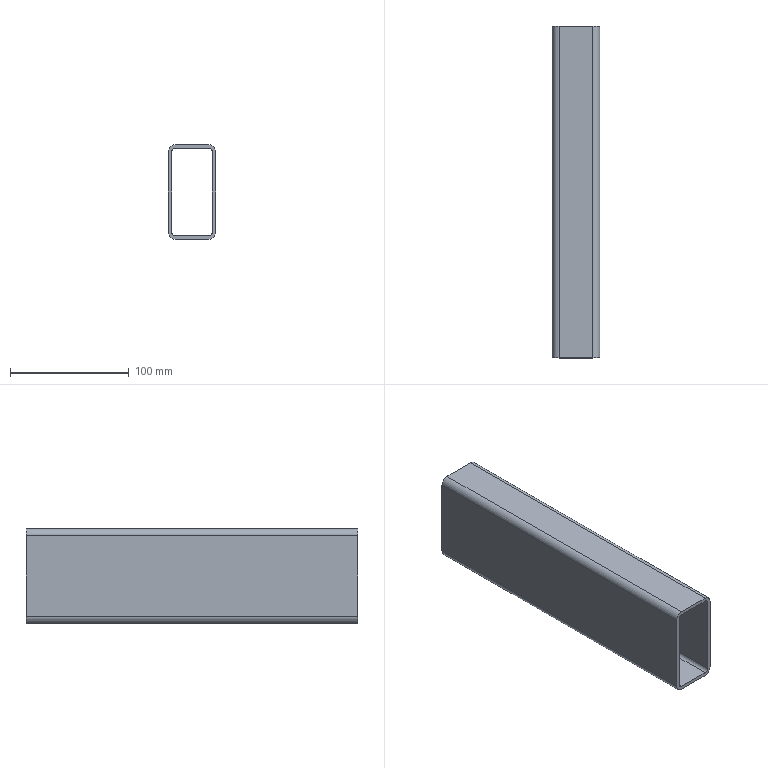Part | STEP file | SN10_002_008-06_TUBO_RETANGULAR | 1 solid | 18 faces | box 40 x 280 x 80 mm | volume 185030 mm3 | plane 10 | cylinder 8 | commonest cylinder face diameters 6 x4 12 x4
STEP:
#1=CARTESIAN_POINT('',(0.,0.,0.));
#2=DIRECTION('',(0.,0.,1.));
#3=DIRECTION('',(1.,0.,0.));
#4=AXIS2_PLACEMENT_3D('',#1,#2,#3);
#5=CARTESIAN_POINT('',(14.,-140.,40.));
#6=VERTEX_POINT('',#5);
#7=CARTESIAN_POINT('',(14.,140.,40.));
#8=VERTEX_POINT('',#7);
#9=CARTESIAN_POINT('',(14.,-140.,40.));
#10=DIRECTION('',(0.,1.,0.));
#11=VECTOR('',#10,1.);
#12=LINE('',#9,#11);
#13=CARTESIAN_POINT('',(14.,0.,34.));
#14=DIRECTION('',(0.,1.,0.));
#15=DIRECTION('',(0.,0.,1.));
#16=AXIS2_PLACEMENT_3D('',#13,#14,#15);
#17=CYLINDRICAL_SURFACE('',#16,6.);
#18=CARTESIAN_POINT('',(0.,-140.));
#19=DIRECTION('',(0.,1.));
#20=VECTOR('',#19,1.);
#21=LINE('',#18,#20);
#22=(GEOMETRIC_REPRESENTATION_CONTEXT(2)PARAMETRIC_REPRESENTATION_CONTEXT()REPRESENTATION_CONTEXT('',''));
#23=DEFINITIONAL_REPRESENTATION('',(#21),#22);
#24=PCURVE('',#17,#23);
#25=CARTESIAN_POINT('',(14.,0.,40.));
#26=DIRECTION('',(0.,0.,-1.));
#27=DIRECTION('',(-1.,0.,0.));
#28=AXIS2_PLACEMENT_3D('',#25,#26,#27);
#29=PLANE('',#28);
#30=CARTESIAN_POINT('',(0.,-140.));
#31=DIRECTION('',(0.,1.));
#32=VECTOR('',#31,1.);
#33=LINE('',#30,#32);
#34=(GEOMETRIC_REPRESENTATION_CONTEXT(2)PARAMETRIC_REPRESENTATION_CONTEXT()REPRESENTATION_CONTEXT('',''));
#35=DEFINITIONAL_REPRESENTATION('',(#33),#34);
#36=PCURVE('',#29,#35);
#37=SURFACE_CURVE('',#12,(#24,#36),.PCURVE_S1.);
#38=EDGE_CURVE('',#6,#8,#37,.T.);
#39=ORIENTED_EDGE('',*,*,#38,.F.);
#40=CARTESIAN_POINT('',(20.,-140.,34.));
#41=VERTEX_POINT('',#40);
#42=CARTESIAN_POINT('',(14.,-140.,34.));
#43=DIRECTION('',(0.,1.,0.));
#44=DIRECTION('',(1.,0.,0.));
#45=AXIS2_PLACEMENT_3D('',#42,#43,#44);
#46=CIRCLE('',#45,6.);
#47=CARTESIAN_POINT('',(-4.712,-140.));
#48=DIRECTION('',(1.,0.));
#49=VECTOR('',#48,1.);
#50=LINE('',#47,#49);
#51=(GEOMETRIC_REPRESENTATION_CONTEXT(2)PARAMETRIC_REPRESENTATION_CONTEXT()REPRESENTATION_CONTEXT('',''));
#52=DEFINITIONAL_REPRESENTATION('',(#50),#51);
#53=PCURVE('',#17,#52);
#54=CARTESIAN_POINT('',(0.,-140.,0.));
#55=DIRECTION('',(0.,1.,0.));
#56=DIRECTION('',(0.,0.,1.));
#57=AXIS2_PLACEMENT_3D('',#54,#55,#56);
#58=PLANE('',#57);
#59=CARTESIAN_POINT('',(34.,14.));
#60=DIRECTION('',(0.,1.));
#61=AXIS2_PLACEMENT_2D('',#59,#60);
#62=CIRCLE('',#61,6.);
#63=(GEOMETRIC_REPRESENTATION_CONTEXT(2)PARAMETRIC_REPRESENTATION_CONTEXT()REPRESENTATION_CONTEXT('',''));
#64=DEFINITIONAL_REPRESENTATION('',(#62),#63);
#65=PCURVE('',#58,#64);
#66=SURFACE_CURVE('',#46,(#53,#65),.PCURVE_S1.);
#67=EDGE_CURVE('',#6,#41,#66,.T.);
#68=ORIENTED_EDGE('',*,*,#67,.T.);
#69=CARTESIAN_POINT('',(20.,140.,34.));
#70=VERTEX_POINT('',#69);
#71=CARTESIAN_POINT('',(20.,-140.,34.));
#72=DIRECTION('',(0.,1.,0.));
#73=VECTOR('',#72,1.);
#74=LINE('',#71,#73);
#75=CARTESIAN_POINT('',(1.571,-140.));
#76=DIRECTION('',(0.,1.));
#77=VECTOR('',#76,1.);
#78=LINE('',#75,#77);
#79=(GEOMETRIC_REPRESENTATION_CONTEXT(2)PARAMETRIC_REPRESENTATION_CONTEXT()REPRESENTATION_CONTEXT('',''));
#80=DEFINITIONAL_REPRESENTATION('',(#78),#79);
#81=PCURVE('',#17,#80);
#82=CARTESIAN_POINT('',(20.,0.,-34.));
#83=DIRECTION('',(-1.,0.,0.));
#84=DIRECTION('',(0.,0.,1.));
#85=AXIS2_PLACEMENT_3D('',#82,#83,#84);
#86=PLANE('',#85);
#87=CARTESIAN_POINT('',(68.,-140.));
#88=DIRECTION('',(0.,1.));
#89=VECTOR('',#88,1.);
#90=LINE('',#87,#89);
#91=(GEOMETRIC_REPRESENTATION_CONTEXT(2)PARAMETRIC_REPRESENTATION_CONTEXT()REPRESENTATION_CONTEXT('',''));
#92=DEFINITIONAL_REPRESENTATION('',(#90),#91);
#93=PCURVE('',#86,#92);
#94=SURFACE_CURVE('',#74,(#81,#93),.PCURVE_S1.);
#95=EDGE_CURVE('',#41,#70,#94,.T.);
#96=ORIENTED_EDGE('',*,*,#95,.T.);
#97=CARTESIAN_POINT('',(14.,140.,34.));
#98=DIRECTION('',(0.,1.,0.));
#99=DIRECTION('',(1.,0.,0.));
#100=AXIS2_PLACEMENT_3D('',#97,#98,#99);
#101=CIRCLE('',#100,6.);
#102=CARTESIAN_POINT('',(-4.712,140.));
#103=DIRECTION('',(1.,0.));
#104=VECTOR('',#103,1.);
#105=LINE('',#102,#104);
#106=(GEOMETRIC_REPRESENTATION_CONTEXT(2)PARAMETRIC_REPRESENTATION_CONTEXT()REPRESENTATION_CONTEXT('',''));
#107=DEFINITIONAL_REPRESENTATION('',(#105),#106);
#108=PCURVE('',#17,#107);
#109=CARTESIAN_POINT('',(0.,140.,0.));
#110=DIRECTION('',(0.,1.,0.));
#111=DIRECTION('',(0.,0.,1.));
#112=AXIS2_PLACEMENT_3D('',#109,#110,#111);
#113=PLANE('',#112);
#114=CARTESIAN_POINT('',(34.,14.));
#115=DIRECTION('',(0.,1.));
#116=AXIS2_PLACEMENT_2D('',#114,#115);
#117=CIRCLE('',#116,6.);
#118=(GEOMETRIC_REPRESENTATION_CONTEXT(2)PARAMETRIC_REPRESENTATION_CONTEXT()REPRESENTATION_CONTEXT('',''));
#119=DEFINITIONAL_REPRESENTATION('',(#117),#118);
#120=PCURVE('',#113,#119);
#121=SURFACE_CURVE('',#101,(#108,#120),.PCURVE_S1.);
#122=EDGE_CURVE('',#8,#70,#121,.T.);
#123=ORIENTED_EDGE('',*,*,#122,.F.);
#124=EDGE_LOOP('',(#39,#68,#96,#123));
#125=FACE_BOUND('',#124,.T.);
#126=ADVANCED_FACE('',(#125),#17,.T.);
#127=ORIENTED_EDGE('',*,*,#95,.F.);
#128=CARTESIAN_POINT('',(20.,-140.,-34.));
#129=VERTEX_POINT('',#128);
#130=CARTESIAN_POINT('',(20.,-140.,-34.));
#131=DIRECTION('',(0.,0.,1.));
#132=VECTOR('',#131,1.);
#133=LINE('',#130,#132);
#134=CARTESIAN_POINT('',(0.,-140.));
#135=DIRECTION('',(1.,0.));
#136=VECTOR('',#135,1.);
#137=LINE('',#134,#136);
#138=(GEOMETRIC_REPRESENTATION_CONTEXT(2)PARAMETRIC_REPRESENTATION_CONTEXT()REPRESENTATION_CONTEXT('',''));
#139=DEFINITIONAL_REPRESENTATION('',(#137),#138);
#140=PCURVE('',#86,#139);
#141=CARTESIAN_POINT('',(-34.,20.));
#142=DIRECTION('',(1.,0.));
#143=VECTOR('',#142,1.);
#144=LINE('',#141,#143);
#145=(GEOMETRIC_REPRESENTATION_CONTEXT(2)PARAMETRIC_REPRESENTATION_CONTEXT()REPRESENTATION_CONTEXT('',''));
#146=DEFINITIONAL_REPRESENTATION('',(#144),#145);
#147=PCURVE('',#58,#146);
#148=SURFACE_CURVE('',#133,(#140,#147),.PCURVE_S1.);
#149=EDGE_CURVE('',#129,#41,#148,.T.);
#150=ORIENTED_EDGE('',*,*,#149,.F.);
#151=CARTESIAN_POINT('',(20.,140.,-34.));
#152=VERTEX_POINT('',#151);
#153=CARTESIAN_POINT('',(20.,-140.,-34.));
#154=DIRECTION('',(0.,1.,0.));
#155=VECTOR('',#154,1.);
#156=LINE('',#153,#155);
#157=CARTESIAN_POINT('',(0.,-140.));
#158=DIRECTION('',(0.,1.));
#159=VECTOR('',#158,1.);
#160=LINE('',#157,#159);
#161=(GEOMETRIC_REPRESENTATION_CONTEXT(2)PARAMETRIC_REPRESENTATION_CONTEXT()REPRESENTATION_CONTEXT('',''));
#162=DEFINITIONAL_REPRESENTATION('',(#160),#161);
#163=PCURVE('',#86,#162);
#164=CARTESIAN_POINT('',(14.,0.,-34.));
#165=DIRECTION('',(0.,1.,0.));
#166=DIRECTION('',(1.,0.,0.));
#167=AXIS2_PLACEMENT_3D('',#164,#165,#166);
#168=CYLINDRICAL_SURFACE('',#167,6.);
#169=CARTESIAN_POINT('',(0.,-140.));
#170=DIRECTION('',(0.,1.));
#171=VECTOR('',#170,1.);
#172=LINE('',#169,#171);
#173=(GEOMETRIC_REPRESENTATION_CONTEXT(2)PARAMETRIC_REPRESENTATION_CONTEXT()REPRESENTATION_CONTEXT('',''));
#174=DEFINITIONAL_REPRESENTATION('',(#172),#173);
#175=PCURVE('',#168,#174);
#176=SURFACE_CURVE('',#156,(#163,#175),.PCURVE_S1.);
#177=EDGE_CURVE('',#129,#152,#176,.T.);
#178=ORIENTED_EDGE('',*,*,#177,.T.);
#179=CARTESIAN_POINT('',(20.,140.,-34.));
#180=DIRECTION('',(0.,0.,1.));
#181=VECTOR('',#180,1.);
#182=LINE('',#179,#181);
#183=CARTESIAN_POINT('',(0.,140.));
#184=DIRECTION('',(1.,0.));
#185=VECTOR('',#184,1.);
#186=LINE('',#183,#185);
#187=(GEOMETRIC_REPRESENTATION_CONTEXT(2)PARAMETRIC_REPRESENTATION_CONTEXT()REPRESENTATION_CONTEXT('',''));
#188=DEFINITIONAL_REPRESENTATION('',(#186),#187);
#189=PCURVE('',#86,#188);
#190=CARTESIAN_POINT('',(-34.,20.));
#191=DIRECTION('',(1.,0.));
#192=VECTOR('',#191,1.);
#193=LINE('',#190,#192);
#194=(GEOMETRIC_REPRESENTATION_CONTEXT(2)PARAMETRIC_REPRESENTATION_CONTEXT()REPRESENTATION_CONTEXT('',''));
#195=DEFINITIONAL_REPRESENTATION('',(#193),#194);
#196=PCURVE('',#113,#195);
#197=SURFACE_CURVE('',#182,(#189,#196),.PCURVE_S1.);
#198=EDGE_CURVE('',#152,#70,#197,.T.);
#199=ORIENTED_EDGE('',*,*,#198,.T.);
#200=EDGE_LOOP('',(#127,#150,#178,#199));
#201=FACE_BOUND('',#200,.T.);
#202=ADVANCED_FACE('',(#201),#86,.F.);
#203=ORIENTED_EDGE('',*,*,#177,.F.);
#204=CARTESIAN_POINT('',(14.,-140.,-40.));
#205=VERTEX_POINT('',#204);
#206=CARTESIAN_POINT('',(14.,-140.,-34.));
#207=DIRECTION('',(0.,1.,0.));
#208=DIRECTION('',(1.,0.,0.));
#209=AXIS2_PLACEMENT_3D('',#206,#207,#208);
#210=CIRCLE('',#209,6.);
#211=CARTESIAN_POINT('',(0.,-140.));
#212=DIRECTION('',(1.,0.));
#213=VECTOR('',#212,1.);
#214=LINE('',#211,#213);
#215=(GEOMETRIC_REPRESENTATION_CONTEXT(2)PARAMETRIC_REPRESENTATION_CONTEXT()REPRESENTATION_CONTEXT('',''));
#216=DEFINITIONAL_REPRESENTATION('',(#214),#215);
#217=PCURVE('',#168,#216);
#218=CARTESIAN_POINT('',(-34.,14.));
#219=DIRECTION('',(0.,1.));
#220=AXIS2_PLACEMENT_2D('',#218,#219);
#221=CIRCLE('',#220,6.);
#222=(GEOMETRIC_REPRESENTATION_CONTEXT(2)PARAMETRIC_REPRESENTATION_CONTEXT()REPRESENTATION_CONTEXT('',''));
#223=DEFINITIONAL_REPRESENTATION('',(#221),#222);
#224=PCURVE('',#58,#223);
#225=SURFACE_CURVE('',#210,(#217,#224),.PCURVE_S1.);
#226=EDGE_CURVE('',#129,#205,#225,.T.);
#227=ORIENTED_EDGE('',*,*,#226,.T.);
#228=CARTESIAN_POINT('',(14.,140.,-40.));
#229=VERTEX_POINT('',#228);
#230=CARTESIAN_POINT('',(14.,-140.,-40.));
#231=DIRECTION('',(0.,1.,0.));
#232=VECTOR('',#231,1.);
#233=LINE('',#230,#232);
#234=CARTESIAN_POINT('',(1.571,-140.));
#235=DIRECTION('',(0.,1.));
#236=VECTOR('',#235,1.);
#237=LINE('',#234,#236);
#238=(GEOMETRIC_REPRESENTATION_CONTEXT(2)PARAMETRIC_REPRESENTATION_CONTEXT()REPRESENTATION_CONTEXT('',''));
#239=DEFINITIONAL_REPRESENTATION('',(#237),#238);
#240=PCURVE('',#168,#239);
#241=CARTESIAN_POINT('',(-14.,0.,-40.));
#242=DIRECTION('',(0.,0.,1.));
#243=DIRECTION('',(1.,0.,0.));
#244=AXIS2_PLACEMENT_3D('',#241,#242,#243);
#245=PLANE('',#244);
#246=CARTESIAN_POINT('',(28.,-140.));
#247=DIRECTION('',(0.,1.));
#248=VECTOR('',#247,1.);
#249=LINE('',#246,#248);
#250=(GEOMETRIC_REPRESENTATION_CONTEXT(2)PARAMETRIC_REPRESENTATION_CONTEXT()REPRESENTATION_CONTEXT('',''));
#251=DEFINITIONAL_REPRESENTATION('',(#249),#250);
#252=PCURVE('',#245,#251);
#253=SURFACE_CURVE('',#233,(#240,#252),.PCURVE_S1.);
#254=EDGE_CURVE('',#205,#229,#253,.T.);
#255=ORIENTED_EDGE('',*,*,#254,.T.);
#256=CARTESIAN_POINT('',(14.,140.,-34.));
#257=DIRECTION('',(0.,1.,0.));
#258=DIRECTION('',(1.,0.,0.));
#259=AXIS2_PLACEMENT_3D('',#256,#257,#258);
#260=CIRCLE('',#259,6.);
#261=CARTESIAN_POINT('',(0.,140.));
#262=DIRECTION('',(1.,0.));
#263=VECTOR('',#262,1.);
#264=LINE('',#261,#263);
#265=(GEOMETRIC_REPRESENTATION_CONTEXT(2)PARAMETRIC_REPRESENTATION_CONTEXT()REPRESENTATION_CONTEXT('',''));
#266=DEFINITIONAL_REPRESENTATION('',(#264),#265);
#267=PCURVE('',#168,#266);
#268=CARTESIAN_POINT('',(-34.,14.));
#269=DIRECTION('',(0.,1.));
#270=AXIS2_PLACEMENT_2D('',#268,#269);
#271=CIRCLE('',#270,6.);
#272=(GEOMETRIC_REPRESENTATION_CONTEXT(2)PARAMETRIC_REPRESENTATION_CONTEXT()REPRESENTATION_CONTEXT('',''));
#273=DEFINITIONAL_REPRESENTATION('',(#271),#272);
#274=PCURVE('',#113,#273);
#275=SURFACE_CURVE('',#260,(#267,#274),.PCURVE_S1.);
#276=EDGE_CURVE('',#152,#229,#275,.T.);
#277=ORIENTED_EDGE('',*,*,#276,.F.);
#278=EDGE_LOOP('',(#203,#227,#255,#277));
#279=FACE_BOUND('',#278,.T.);
#280=ADVANCED_FACE('',(#279),#168,.T.);
#281=ORIENTED_EDGE('',*,*,#254,.F.);
#282=CARTESIAN_POINT('',(-14.,-140.,-40.));
#283=VERTEX_POINT('',#282);
#284=CARTESIAN_POINT('',(-14.,-140.,-40.));
#285=DIRECTION('',(1.,0.,0.));
#286=VECTOR('',#285,1.);
#287=LINE('',#284,#286);
#288=CARTESIAN_POINT('',(0.,-140.));
#289=DIRECTION('',(1.,0.));
#290=VECTOR('',#289,1.);
#291=LINE('',#288,#290);
#292=(GEOMETRIC_REPRESENTATION_CONTEXT(2)PARAMETRIC_REPRESENTATION_CONTEXT()REPRESENTATION_CONTEXT('',''));
#293=DEFINITIONAL_REPRESENTATION('',(#291),#292);
#294=PCURVE('',#245,#293);
#295=CARTESIAN_POINT('',(-40.,-14.));
#296=DIRECTION('',(0.,1.));
#297=VECTOR('',#296,1.);
#298=LINE('',#295,#297);
#299=(GEOMETRIC_REPRESENTATION_CONTEXT(2)PARAMETRIC_REPRESENTATION_CONTEXT()REPRESENTATION_CONTEXT('',''));
#300=DEFINITIONAL_REPRESENTATION('',(#298),#299);
#301=PCURVE('',#58,#300);
#302=SURFACE_CURVE('',#287,(#294,#301),.PCURVE_S1.);
#303=EDGE_CURVE('',#283,#205,#302,.T.);
#304=ORIENTED_EDGE('',*,*,#303,.F.);
#305=CARTESIAN_POINT('',(-14.,140.,-40.));
#306=VERTEX_POINT('',#305);
#307=CARTESIAN_POINT('',(-14.,-140.,-40.));
#308=DIRECTION('',(0.,1.,0.));
#309=VECTOR('',#308,1.);
#310=LINE('',#307,#309);
#311=CARTESIAN_POINT('',(0.,-140.));
#312=DIRECTION('',(0.,1.));
#313=VECTOR('',#312,1.);
#314=LINE('',#311,#313);
#315=(GEOMETRIC_REPRESENTATION_CONTEXT(2)PARAMETRIC_REPRESENTATION_CONTEXT()REPRESENTATION_CONTEXT('',''));
#316=DEFINITIONAL_REPRESENTATION('',(#314),#315);
#317=PCURVE('',#245,#316);
#318=CARTESIAN_POINT('',(-14.,0.,-34.));
#319=DIRECTION('',(0.,1.,0.));
#320=DIRECTION('',(0.,0.,-1.));
#321=AXIS2_PLACEMENT_3D('',#318,#319,#320);
#322=CYLINDRICAL_SURFACE('',#321,6.);
#323=CARTESIAN_POINT('',(0.,-140.));
#324=DIRECTION('',(0.,1.));
#325=VECTOR('',#324,1.);
#326=LINE('',#323,#325);
#327=(GEOMETRIC_REPRESENTATION_CONTEXT(2)PARAMETRIC_REPRESENTATION_CONTEXT()REPRESENTATION_CONTEXT('',''));
#328=DEFINITIONAL_REPRESENTATION('',(#326),#327);
#329=PCURVE('',#322,#328);
#330=SURFACE_CURVE('',#310,(#317,#329),.PCURVE_S1.);
#331=EDGE_CURVE('',#283,#306,#330,.T.);
#332=ORIENTED_EDGE('',*,*,#331,.T.);
#333=CARTESIAN_POINT('',(-14.,140.,-40.));
#334=DIRECTION('',(1.,0.,0.));
#335=VECTOR('',#334,1.);
#336=LINE('',#333,#335);
#337=CARTESIAN_POINT('',(0.,140.));
#338=DIRECTION('',(1.,0.));
#339=VECTOR('',#338,1.);
#340=LINE('',#337,#339);
#341=(GEOMETRIC_REPRESENTATION_CONTEXT(2)PARAMETRIC_REPRESENTATION_CONTEXT()REPRESENTATION_CONTEXT('',''));
#342=DEFINITIONAL_REPRESENTATION('',(#340),#341);
#343=PCURVE('',#245,#342);
#344=CARTESIAN_POINT('',(-40.,-14.));
#345=DIRECTION('',(0.,1.));
#346=VECTOR('',#345,1.);
#347=LINE('',#344,#346);
#348=(GEOMETRIC_REPRESENTATION_CONTEXT(2)PARAMETRIC_REPRESENTATION_CONTEXT()REPRESENTATION_CONTEXT('',''));
#349=DEFINITIONAL_REPRESENTATION('',(#347),#348);
#350=PCURVE('',#113,#349);
#351=SURFACE_CURVE('',#336,(#343,#350),.PCURVE_S1.);
#352=EDGE_CURVE('',#306,#229,#351,.T.);
#353=ORIENTED_EDGE('',*,*,#352,.T.);
#354=EDGE_LOOP('',(#281,#304,#332,#353));
#355=FACE_BOUND('',#354,.T.);
#356=ADVANCED_FACE('',(#355),#245,.F.);
#357=ORIENTED_EDGE('',*,*,#331,.F.);
#358=CARTESIAN_POINT('',(-20.,-140.,-34.));
#359=VERTEX_POINT('',#358);
#360=CARTESIAN_POINT('',(-14.,-140.,-34.));
#361=DIRECTION('',(0.,1.,0.));
#362=DIRECTION('',(1.,0.,0.));
#363=AXIS2_PLACEMENT_3D('',#360,#361,#362);
#364=CIRCLE('',#363,6.);
#365=CARTESIAN_POINT('',(-1.571,-140.));
#366=DIRECTION('',(1.,0.));
#367=VECTOR('',#366,1.);
#368=LINE('',#365,#367);
#369=(GEOMETRIC_REPRESENTATION_CONTEXT(2)PARAMETRIC_REPRESENTATION_CONTEXT()REPRESENTATION_CONTEXT('',''));
#370=DEFINITIONAL_REPRESENTATION('',(#368),#369);
#371=PCURVE('',#322,#370);
#372=CARTESIAN_POINT('',(-34.,-14.));
#373=DIRECTION('',(0.,1.));
#374=AXIS2_PLACEMENT_2D('',#372,#373);
#375=CIRCLE('',#374,6.);
#376=(GEOMETRIC_REPRESENTATION_CONTEXT(2)PARAMETRIC_REPRESENTATION_CONTEXT()REPRESENTATION_CONTEXT('',''));
#377=DEFINITIONAL_REPRESENTATION('',(#375),#376);
#378=PCURVE('',#58,#377);
#379=SURFACE_CURVE('',#364,(#371,#378),.PCURVE_S1.);
#380=EDGE_CURVE('',#283,#359,#379,.T.);
#381=ORIENTED_EDGE('',*,*,#380,.T.);
#382=CARTESIAN_POINT('',(-20.,140.,-34.));
#383=VERTEX_POINT('',#382);
#384=CARTESIAN_POINT('',(-20.,-140.,-34.));
#385=DIRECTION('',(0.,1.,0.));
#386=VECTOR('',#385,1.);
#387=LINE('',#384,#386);
#388=CARTESIAN_POINT('',(1.571,-140.));
#389=DIRECTION('',(0.,1.));
#390=VECTOR('',#389,1.);
#391=LINE('',#388,#390);
#392=(GEOMETRIC_REPRESENTATION_CONTEXT(2)PARAMETRIC_REPRESENTATION_CONTEXT()REPRESENTATION_CONTEXT('',''));
#393=DEFINITIONAL_REPRESENTATION('',(#391),#392);
#394=PCURVE('',#322,#393);
#395=CARTESIAN_POINT('',(-20.,0.,34.));
#396=DIRECTION('',(1.,0.,0.));
#397=DIRECTION('',(0.,0.,-1.));
#398=AXIS2_PLACEMENT_3D('',#395,#396,#397);
#399=PLANE('',#398);
#400=CARTESIAN_POINT('',(68.,-140.));
#401=DIRECTION('',(0.,1.));
#402=VECTOR('',#401,1.);
#403=LINE('',#400,#402);
#404=(GEOMETRIC_REPRESENTATION_CONTEXT(2)PARAMETRIC_REPRESENTATION_CONTEXT()REPRESENTATION_CONTEXT('',''));
#405=DEFINITIONAL_REPRESENTATION('',(#403),#404);
#406=PCURVE('',#399,#405);
#407=SURFACE_CURVE('',#387,(#394,#406),.PCURVE_S1.);
#408=EDGE_CURVE('',#359,#383,#407,.T.);
#409=ORIENTED_EDGE('',*,*,#408,.T.);
#410=CARTESIAN_POINT('',(-14.,140.,-34.));
#411=DIRECTION('',(0.,1.,0.));
#412=DIRECTION('',(1.,0.,0.));
#413=AXIS2_PLACEMENT_3D('',#410,#411,#412);
#414=CIRCLE('',#413,6.);
#415=CARTESIAN_POINT('',(-1.571,140.));
#416=DIRECTION('',(1.,0.));
#417=VECTOR('',#416,1.);
#418=LINE('',#415,#417);
#419=(GEOMETRIC_REPRESENTATION_CONTEXT(2)PARAMETRIC_REPRESENTATION_CONTEXT()REPRESENTATION_CONTEXT('',''));
#420=DEFINITIONAL_REPRESENTATION('',(#418),#419);
#421=PCURVE('',#322,#420);
#422=CARTESIAN_POINT('',(-34.,-14.));
#423=DIRECTION('',(0.,1.));
#424=AXIS2_PLACEMENT_2D('',#422,#423);
#425=CIRCLE('',#424,6.);
#426=(GEOMETRIC_REPRESENTATION_CONTEXT(2)PARAMETRIC_REPRESENTATION_CONTEXT()REPRESENTATION_CONTEXT('',''));
#427=DEFINITIONAL_REPRESENTATION('',(#425),#426);
#428=PCURVE('',#113,#427);
#429=SURFACE_CURVE('',#414,(#421,#428),.PCURVE_S1.);
#430=EDGE_CURVE('',#306,#383,#429,.T.);
#431=ORIENTED_EDGE('',*,*,#430,.F.);
#432=EDGE_LOOP('',(#357,#381,#409,#431));
#433=FACE_BOUND('',#432,.T.);
#434=ADVANCED_FACE('',(#433),#322,.T.);
#435=ORIENTED_EDGE('',*,*,#408,.F.);
#436=CARTESIAN_POINT('',(-20.,-140.,34.));
#437=VERTEX_POINT('',#436);
#438=CARTESIAN_POINT('',(-20.,-140.,34.));
#439=DIRECTION('',(0.,0.,-1.));
#440=VECTOR('',#439,1.);
#441=LINE('',#438,#440);
#442=CARTESIAN_POINT('',(0.,-140.));
#443=DIRECTION('',(1.,0.));
#444=VECTOR('',#443,1.);
#445=LINE('',#442,#444);
#446=(GEOMETRIC_REPRESENTATION_CONTEXT(2)PARAMETRIC_REPRESENTATION_CONTEXT()REPRESENTATION_CONTEXT('',''));
#447=DEFINITIONAL_REPRESENTATION('',(#445),#446);
#448=PCURVE('',#399,#447);
#449=CARTESIAN_POINT('',(34.,-20.));
#450=DIRECTION('',(-1.,0.));
#451=VECTOR('',#450,1.);
#452=LINE('',#449,#451);
#453=(GEOMETRIC_REPRESENTATION_CONTEXT(2)PARAMETRIC_REPRESENTATION_CONTEXT()REPRESENTATION_CONTEXT('',''));
#454=DEFINITIONAL_REPRESENTATION('',(#452),#453);
#455=PCURVE('',#58,#454);
#456=SURFACE_CURVE('',#441,(#448,#455),.PCURVE_S1.);
#457=EDGE_CURVE('',#437,#359,#456,.T.);
#458=ORIENTED_EDGE('',*,*,#457,.F.);
#459=CARTESIAN_POINT('',(-20.,140.,34.));
#460=VERTEX_POINT('',#459);
#461=CARTESIAN_POINT('',(-20.,-140.,34.));
#462=DIRECTION('',(0.,1.,0.));
#463=VECTOR('',#462,1.);
#464=LINE('',#461,#463);
#465=CARTESIAN_POINT('',(0.,-140.));
#466=DIRECTION('',(0.,1.));
#467=VECTOR('',#466,1.);
#468=LINE('',#465,#467);
#469=(GEOMETRIC_REPRESENTATION_CONTEXT(2)PARAMETRIC_REPRESENTATION_CONTEXT()REPRESENTATION_CONTEXT('',''));
#470=DEFINITIONAL_REPRESENTATION('',(#468),#469);
#471=PCURVE('',#399,#470);
#472=CARTESIAN_POINT('',(-14.,0.,34.));
#473=DIRECTION('',(0.,1.,0.));
#474=DIRECTION('',(-1.,0.,0.));
#475=AXIS2_PLACEMENT_3D('',#472,#473,#474);
#476=CYLINDRICAL_SURFACE('',#475,6.);
#477=CARTESIAN_POINT('',(0.,-140.));
#478=DIRECTION('',(0.,1.));
#479=VECTOR('',#478,1.);
#480=LINE('',#477,#479);
#481=(GEOMETRIC_REPRESENTATION_CONTEXT(2)PARAMETRIC_REPRESENTATION_CONTEXT()REPRESENTATION_CONTEXT('',''));
#482=DEFINITIONAL_REPRESENTATION('',(#480),#481);
#483=PCURVE('',#476,#482);
#484=SURFACE_CURVE('',#464,(#471,#483),.PCURVE_S1.);
#485=EDGE_CURVE('',#437,#460,#484,.T.);
#486=ORIENTED_EDGE('',*,*,#485,.T.);
#487=CARTESIAN_POINT('',(-20.,140.,34.));
#488=DIRECTION('',(0.,0.,-1.));
#489=VECTOR('',#488,1.);
#490=LINE('',#487,#489);
#491=CARTESIAN_POINT('',(0.,140.));
#492=DIRECTION('',(1.,0.));
#493=VECTOR('',#492,1.);
#494=LINE('',#491,#493);
#495=(GEOMETRIC_REPRESENTATION_CONTEXT(2)PARAMETRIC_REPRESENTATION_CONTEXT()REPRESENTATION_CONTEXT('',''));
#496=DEFINITIONAL_REPRESENTATION('',(#494),#495);
#497=PCURVE('',#399,#496);
#498=CARTESIAN_POINT('',(34.,-20.));
#499=DIRECTION('',(-1.,0.));
#500=VECTOR('',#499,1.);
#501=LINE('',#498,#500);
#502=(GEOMETRIC_REPRESENTATION_CONTEXT(2)PARAMETRIC_REPRESENTATION_CONTEXT()REPRESENTATION_CONTEXT('',''));
#503=DEFINITIONAL_REPRESENTATION('',(#501),#502);
#504=PCURVE('',#113,#503);
#505=SURFACE_CURVE('',#490,(#497,#504),.PCURVE_S1.);
#506=EDGE_CURVE('',#460,#383,#505,.T.);
#507=ORIENTED_EDGE('',*,*,#506,.T.);
#508=EDGE_LOOP('',(#435,#458,#486,#507));
#509=FACE_BOUND('',#508,.T.);
#510=ADVANCED_FACE('',(#509),#399,.F.);
#511=ORIENTED_EDGE('',*,*,#485,.F.);
#512=CARTESIAN_POINT('',(-14.,-140.,40.));
#513=VERTEX_POINT('',#512);
#514=CARTESIAN_POINT('',(-14.,-140.,34.));
#515=DIRECTION('',(0.,1.,0.));
#516=DIRECTION('',(1.,0.,0.));
#517=AXIS2_PLACEMENT_3D('',#514,#515,#516);
#518=CIRCLE('',#517,6.);
#519=CARTESIAN_POINT('',(-3.142,-140.));
#520=DIRECTION('',(1.,0.));
#521=VECTOR('',#520,1.);
#522=LINE('',#519,#521);
#523=(GEOMETRIC_REPRESENTATION_CONTEXT(2)PARAMETRIC_REPRESENTATION_CONTEXT()REPRESENTATION_CONTEXT('',''));
#524=DEFINITIONAL_REPRESENTATION('',(#522),#523);
#525=PCURVE('',#476,#524);
#526=CARTESIAN_POINT('',(34.,-14.));
#527=DIRECTION('',(0.,1.));
#528=AXIS2_PLACEMENT_2D('',#526,#527);
#529=CIRCLE('',#528,6.);
#530=(GEOMETRIC_REPRESENTATION_CONTEXT(2)PARAMETRIC_REPRESENTATION_CONTEXT()REPRESENTATION_CONTEXT('',''));
#531=DEFINITIONAL_REPRESENTATION('',(#529),#530);
#532=PCURVE('',#58,#531);
#533=SURFACE_CURVE('',#518,(#525,#532),.PCURVE_S1.);
#534=EDGE_CURVE('',#437,#513,#533,.T.);
#535=ORIENTED_EDGE('',*,*,#534,.T.);
#536=CARTESIAN_POINT('',(-14.,140.,40.));
#537=VERTEX_POINT('',#536);
#538=CARTESIAN_POINT('',(-14.,-140.,40.));
#539=DIRECTION('',(0.,1.,0.));
#540=VECTOR('',#539,1.);
#541=LINE('',#538,#540);
#542=CARTESIAN_POINT('',(1.571,-140.));
#543=DIRECTION('',(0.,1.));
#544=VECTOR('',#543,1.);
#545=LINE('',#542,#544);
#546=(GEOMETRIC_REPRESENTATION_CONTEXT(2)PARAMETRIC_REPRESENTATION_CONTEXT()REPRESENTATION_CONTEXT('',''));
#547=DEFINITIONAL_REPRESENTATION('',(#545),#546);
#548=PCURVE('',#476,#547);
#549=CARTESIAN_POINT('',(28.,-140.));
#550=DIRECTION('',(0.,1.));
#551=VECTOR('',#550,1.);
#552=LINE('',#549,#551);
#553=(GEOMETRIC_REPRESENTATION_CONTEXT(2)PARAMETRIC_REPRESENTATION_CONTEXT()REPRESENTATION_CONTEXT('',''));
#554=DEFINITIONAL_REPRESENTATION('',(#552),#553);
#555=PCURVE('',#29,#554);
#556=SURFACE_CURVE('',#541,(#548,#555),.PCURVE_S1.);
#557=EDGE_CURVE('',#513,#537,#556,.T.);
#558=ORIENTED_EDGE('',*,*,#557,.T.);
#559=CARTESIAN_POINT('',(-14.,140.,34.));
#560=DIRECTION('',(0.,1.,0.));
#561=DIRECTION('',(1.,0.,0.));
#562=AXIS2_PLACEMENT_3D('',#559,#560,#561);
#563=CIRCLE('',#562,6.);
#564=CARTESIAN_POINT('',(-3.142,140.));
#565=DIRECTION('',(1.,0.));
#566=VECTOR('',#565,1.);
#567=LINE('',#564,#566);
#568=(GEOMETRIC_REPRESENTATION_CONTEXT(2)PARAMETRIC_REPRESENTATION_CONTEXT()REPRESENTATION_CONTEXT('',''));
#569=DEFINITIONAL_REPRESENTATION('',(#567),#568);
#570=PCURVE('',#476,#569);
#571=CARTESIAN_POINT('',(34.,-14.));
#572=DIRECTION('',(0.,1.));
#573=AXIS2_PLACEMENT_2D('',#571,#572);
#574=CIRCLE('',#573,6.);
#575=(GEOMETRIC_REPRESENTATION_CONTEXT(2)PARAMETRIC_REPRESENTATION_CONTEXT()REPRESENTATION_CONTEXT('',''));
#576=DEFINITIONAL_REPRESENTATION('',(#574),#575);
#577=PCURVE('',#113,#576);
#578=SURFACE_CURVE('',#563,(#570,#577),.PCURVE_S1.);
#579=EDGE_CURVE('',#460,#537,#578,.T.);
#580=ORIENTED_EDGE('',*,*,#579,.F.);
#581=EDGE_LOOP('',(#511,#535,#558,#580));
#582=FACE_BOUND('',#581,.T.);
#583=ADVANCED_FACE('',(#582),#476,.T.);
#584=ORIENTED_EDGE('',*,*,#557,.F.);
#585=CARTESIAN_POINT('',(14.,-140.,40.));
#586=DIRECTION('',(-1.,0.,0.));
#587=VECTOR('',#586,1.);
#588=LINE('',#585,#587);
#589=CARTESIAN_POINT('',(0.,-140.));
#590=DIRECTION('',(1.,0.));
#591=VECTOR('',#590,1.);
#592=LINE('',#589,#591);
#593=(GEOMETRIC_REPRESENTATION_CONTEXT(2)PARAMETRIC_REPRESENTATION_CONTEXT()REPRESENTATION_CONTEXT('',''));
#594=DEFINITIONAL_REPRESENTATION('',(#592),#593);
#595=PCURVE('',#29,#594);
#596=CARTESIAN_POINT('',(40.,14.));
#597=DIRECTION('',(0.,-1.));
#598=VECTOR('',#597,1.);
#599=LINE('',#596,#598);
#600=(GEOMETRIC_REPRESENTATION_CONTEXT(2)PARAMETRIC_REPRESENTATION_CONTEXT()REPRESENTATION_CONTEXT('',''));
#601=DEFINITIONAL_REPRESENTATION('',(#599),#600);
#602=PCURVE('',#58,#601);
#603=SURFACE_CURVE('',#588,(#595,#602),.PCURVE_S1.);
#604=EDGE_CURVE('',#6,#513,#603,.T.);
#605=ORIENTED_EDGE('',*,*,#604,.F.);
#606=ORIENTED_EDGE('',*,*,#38,.T.);
#607=CARTESIAN_POINT('',(14.,140.,40.));
#608=DIRECTION('',(-1.,0.,0.));
#609=VECTOR('',#608,1.);
#610=LINE('',#607,#609);
#611=CARTESIAN_POINT('',(0.,140.));
#612=DIRECTION('',(1.,0.));
#613=VECTOR('',#612,1.);
#614=LINE('',#611,#613);
#615=(GEOMETRIC_REPRESENTATION_CONTEXT(2)PARAMETRIC_REPRESENTATION_CONTEXT()REPRESENTATION_CONTEXT('',''));
#616=DEFINITIONAL_REPRESENTATION('',(#614),#615);
#617=PCURVE('',#29,#616);
#618=CARTESIAN_POINT('',(40.,14.));
#619=DIRECTION('',(0.,-1.));
#620=VECTOR('',#619,1.);
#621=LINE('',#618,#620);
#622=(GEOMETRIC_REPRESENTATION_CONTEXT(2)PARAMETRIC_REPRESENTATION_CONTEXT()REPRESENTATION_CONTEXT('',''));
#623=DEFINITIONAL_REPRESENTATION('',(#621),#622);
#624=PCURVE('',#113,#623);
#625=SURFACE_CURVE('',#610,(#617,#624),.PCURVE_S1.);
#626=EDGE_CURVE('',#8,#537,#625,.T.);
#627=ORIENTED_EDGE('',*,*,#626,.T.);
#628=EDGE_LOOP('',(#584,#605,#606,#627));
#629=FACE_BOUND('',#628,.T.);
#630=ADVANCED_FACE('',(#629),#29,.F.);
#631=CARTESIAN_POINT('',(14.,140.,37.));
#632=VERTEX_POINT('',#631);
#633=CARTESIAN_POINT('',(-14.,140.,37.));
#634=VERTEX_POINT('',#633);
#635=CARTESIAN_POINT('',(14.,140.,37.));
#636=DIRECTION('',(-1.,0.,0.));
#637=VECTOR('',#636,1.);
#638=LINE('',#635,#637);
#639=CARTESIAN_POINT('',(14.,0.,37.));
#640=DIRECTION('',(0.,0.,-1.));
#641=DIRECTION('',(-1.,0.,0.));
#642=AXIS2_PLACEMENT_3D('',#639,#640,#641);
#643=PLANE('',#642);
#644=CARTESIAN_POINT('',(0.,140.));
#645=DIRECTION('',(1.,0.));
#646=VECTOR('',#645,1.);
#647=LINE('',#644,#646);
#648=(GEOMETRIC_REPRESENTATION_CONTEXT(2)PARAMETRIC_REPRESENTATION_CONTEXT()REPRESENTATION_CONTEXT('',''));
#649=DEFINITIONAL_REPRESENTATION('',(#647),#648);
#650=PCURVE('',#643,#649);
#651=CARTESIAN_POINT('',(37.,14.));
#652=DIRECTION('',(0.,-1.));
#653=VECTOR('',#652,1.);
#654=LINE('',#651,#653);
#655=(GEOMETRIC_REPRESENTATION_CONTEXT(2)PARAMETRIC_REPRESENTATION_CONTEXT()REPRESENTATION_CONTEXT('',''));
#656=DEFINITIONAL_REPRESENTATION('',(#654),#655);
#657=PCURVE('',#113,#656);
#658=SURFACE_CURVE('',#638,(#650,#657),.PCURVE_S1.);
#659=EDGE_CURVE('',#632,#634,#658,.T.);
#660=ORIENTED_EDGE('',*,*,#659,.F.);
#661=CARTESIAN_POINT('',(14.,-140.,37.));
#662=VERTEX_POINT('',#661);
#663=CARTESIAN_POINT('',(14.,-140.,37.));
#664=DIRECTION('',(0.,1.,0.));
#665=VECTOR('',#664,1.);
#666=LINE('',#663,#665);
#667=CARTESIAN_POINT('',(0.,-140.));
#668=DIRECTION('',(0.,1.));
#669=VECTOR('',#668,1.);
#670=LINE('',#667,#669);
#671=(GEOMETRIC_REPRESENTATION_CONTEXT(2)PARAMETRIC_REPRESENTATION_CONTEXT()REPRESENTATION_CONTEXT('',''));
#672=DEFINITIONAL_REPRESENTATION('',(#670),#671);
#673=PCURVE('',#643,#672);
#674=CARTESIAN_POINT('',(14.,0.,34.));
#675=DIRECTION('',(0.,1.,0.));
#676=DIRECTION('',(0.,0.,1.));
#677=AXIS2_PLACEMENT_3D('',#674,#675,#676);
#678=CYLINDRICAL_SURFACE('',#677,3.);
#679=CARTESIAN_POINT('',(0.,-140.));
#680=DIRECTION('',(0.,1.));
#681=VECTOR('',#680,1.);
#682=LINE('',#679,#681);
#683=(GEOMETRIC_REPRESENTATION_CONTEXT(2)PARAMETRIC_REPRESENTATION_CONTEXT()REPRESENTATION_CONTEXT('',''));
#684=DEFINITIONAL_REPRESENTATION('',(#682),#683);
#685=PCURVE('',#678,#684);
#686=SURFACE_CURVE('',#666,(#673,#685),.PCURVE_S1.);
#687=EDGE_CURVE('',#662,#632,#686,.T.);
#688=ORIENTED_EDGE('',*,*,#687,.F.);
#689=CARTESIAN_POINT('',(-14.,-140.,37.));
#690=VERTEX_POINT('',#689);
#691=CARTESIAN_POINT('',(14.,-140.,37.));
#692=DIRECTION('',(-1.,0.,0.));
#693=VECTOR('',#692,1.);
#694=LINE('',#691,#693);
#695=CARTESIAN_POINT('',(0.,-140.));
#696=DIRECTION('',(1.,0.));
#697=VECTOR('',#696,1.);
#698=LINE('',#695,#697);
#699=(GEOMETRIC_REPRESENTATION_CONTEXT(2)PARAMETRIC_REPRESENTATION_CONTEXT()REPRESENTATION_CONTEXT('',''));
#700=DEFINITIONAL_REPRESENTATION('',(#698),#699);
#701=PCURVE('',#643,#700);
#702=CARTESIAN_POINT('',(37.,14.));
#703=DIRECTION('',(0.,-1.));
#704=VECTOR('',#703,1.);
#705=LINE('',#702,#704);
#706=(GEOMETRIC_REPRESENTATION_CONTEXT(2)PARAMETRIC_REPRESENTATION_CONTEXT()REPRESENTATION_CONTEXT('',''));
#707=DEFINITIONAL_REPRESENTATION('',(#705),#706);
#708=PCURVE('',#58,#707);
#709=SURFACE_CURVE('',#694,(#701,#708),.PCURVE_S1.);
#710=EDGE_CURVE('',#662,#690,#709,.T.);
#711=ORIENTED_EDGE('',*,*,#710,.T.);
#712=CARTESIAN_POINT('',(-14.,-140.,37.));
#713=DIRECTION('',(0.,1.,0.));
#714=VECTOR('',#713,1.);
#715=LINE('',#712,#714);
#716=CARTESIAN_POINT('',(28.,-140.));
#717=DIRECTION('',(0.,1.));
#718=VECTOR('',#717,1.);
#719=LINE('',#716,#718);
#720=(GEOMETRIC_REPRESENTATION_CONTEXT(2)PARAMETRIC_REPRESENTATION_CONTEXT()REPRESENTATION_CONTEXT('',''));
#721=DEFINITIONAL_REPRESENTATION('',(#719),#720);
#722=PCURVE('',#643,#721);
#723=CARTESIAN_POINT('',(-14.,0.,34.));
#724=DIRECTION('',(0.,1.,0.));
#725=DIRECTION('',(-1.,0.,0.));
#726=AXIS2_PLACEMENT_3D('',#723,#724,#725);
#727=CYLINDRICAL_SURFACE('',#726,3.);
#728=CARTESIAN_POINT('',(1.571,-140.));
#729=DIRECTION('',(0.,1.));
#730=VECTOR('',#729,1.);
#731=LINE('',#728,#730);
#732=(GEOMETRIC_REPRESENTATION_CONTEXT(2)PARAMETRIC_REPRESENTATION_CONTEXT()REPRESENTATION_CONTEXT('',''));
#733=DEFINITIONAL_REPRESENTATION('',(#731),#732);
#734=PCURVE('',#727,#733);
#735=SURFACE_CURVE('',#715,(#722,#734),.PCURVE_S1.);
#736=EDGE_CURVE('',#690,#634,#735,.T.);
#737=ORIENTED_EDGE('',*,*,#736,.T.);
#738=EDGE_LOOP('',(#660,#688,#711,#737));
#739=FACE_BOUND('',#738,.T.);
#740=ADVANCED_FACE('',(#739),#643,.T.);
#741=CARTESIAN_POINT('',(-17.,-140.,34.));
#742=VERTEX_POINT('',#741);
#743=CARTESIAN_POINT('',(-17.,140.,34.));
#744=VERTEX_POINT('',#743);
#745=CARTESIAN_POINT('',(-17.,-140.,34.));
#746=DIRECTION('',(0.,1.,0.));
#747=VECTOR('',#746,1.);
#748=LINE('',#745,#747);
#749=CARTESIAN_POINT('',(0.,-140.));
#750=DIRECTION('',(0.,1.));
#751=VECTOR('',#750,1.);
#752=LINE('',#749,#751);
#753=(GEOMETRIC_REPRESENTATION_CONTEXT(2)PARAMETRIC_REPRESENTATION_CONTEXT()REPRESENTATION_CONTEXT('',''));
#754=DEFINITIONAL_REPRESENTATION('',(#752),#753);
#755=PCURVE('',#727,#754);
#756=CARTESIAN_POINT('',(-17.,0.,34.));
#757=DIRECTION('',(1.,0.,0.));
#758=DIRECTION('',(0.,0.,-1.));
#759=AXIS2_PLACEMENT_3D('',#756,#757,#758);
#760=PLANE('',#759);
#761=CARTESIAN_POINT('',(0.,-140.));
#762=DIRECTION('',(0.,1.));
#763=VECTOR('',#762,1.);
#764=LINE('',#761,#763);
#765=(GEOMETRIC_REPRESENTATION_CONTEXT(2)PARAMETRIC_REPRESENTATION_CONTEXT()REPRESENTATION_CONTEXT('',''));
#766=DEFINITIONAL_REPRESENTATION('',(#764),#765);
#767=PCURVE('',#760,#766);
#768=SURFACE_CURVE('',#748,(#755,#767),.PCURVE_S1.);
#769=EDGE_CURVE('',#742,#744,#768,.T.);
#770=ORIENTED_EDGE('',*,*,#769,.F.);
#771=CARTESIAN_POINT('',(-14.,-140.,34.));
#772=DIRECTION('',(0.,1.,0.));
#773=DIRECTION('',(1.,0.,0.));
#774=AXIS2_PLACEMENT_3D('',#771,#772,#773);
#775=CIRCLE('',#774,3.);
#776=CARTESIAN_POINT('',(-3.142,-140.));
#777=DIRECTION('',(1.,0.));
#778=VECTOR('',#777,1.);
#779=LINE('',#776,#778);
#780=(GEOMETRIC_REPRESENTATION_CONTEXT(2)PARAMETRIC_REPRESENTATION_CONTEXT()REPRESENTATION_CONTEXT('',''));
#781=DEFINITIONAL_REPRESENTATION('',(#779),#780);
#782=PCURVE('',#727,#781);
#783=CARTESIAN_POINT('',(34.,-14.));
#784=DIRECTION('',(0.,1.));
#785=AXIS2_PLACEMENT_2D('',#783,#784);
#786=CIRCLE('',#785,3.);
#787=(GEOMETRIC_REPRESENTATION_CONTEXT(2)PARAMETRIC_REPRESENTATION_CONTEXT()REPRESENTATION_CONTEXT('',''));
#788=DEFINITIONAL_REPRESENTATION('',(#786),#787);
#789=PCURVE('',#58,#788);
#790=SURFACE_CURVE('',#775,(#782,#789),.PCURVE_S1.);
#791=EDGE_CURVE('',#742,#690,#790,.T.);
#792=ORIENTED_EDGE('',*,*,#791,.T.);
#793=ORIENTED_EDGE('',*,*,#736,.T.);
#794=CARTESIAN_POINT('',(-14.,140.,34.));
#795=DIRECTION('',(0.,1.,0.));
#796=DIRECTION('',(1.,0.,0.));
#797=AXIS2_PLACEMENT_3D('',#794,#795,#796);
#798=CIRCLE('',#797,3.);
#799=CARTESIAN_POINT('',(-3.142,140.));
#800=DIRECTION('',(1.,0.));
#801=VECTOR('',#800,1.);
#802=LINE('',#799,#801);
#803=(GEOMETRIC_REPRESENTATION_CONTEXT(2)PARAMETRIC_REPRESENTATION_CONTEXT()REPRESENTATION_CONTEXT('',''));
#804=DEFINITIONAL_REPRESENTATION('',(#802),#803);
#805=PCURVE('',#727,#804);
#806=CARTESIAN_POINT('',(34.,-14.));
#807=DIRECTION('',(0.,1.));
#808=AXIS2_PLACEMENT_2D('',#806,#807);
#809=CIRCLE('',#808,3.);
#810=(GEOMETRIC_REPRESENTATION_CONTEXT(2)PARAMETRIC_REPRESENTATION_CONTEXT()REPRESENTATION_CONTEXT('',''));
#811=DEFINITIONAL_REPRESENTATION('',(#809),#810);
#812=PCURVE('',#113,#811);
#813=SURFACE_CURVE('',#798,(#805,#812),.PCURVE_S1.);
#814=EDGE_CURVE('',#744,#634,#813,.T.);
#815=ORIENTED_EDGE('',*,*,#814,.F.);
#816=EDGE_LOOP('',(#770,#792,#793,#815));
#817=FACE_BOUND('',#816,.F.);
#818=ADVANCED_FACE('',(#817),#727,.F.);
#819=CARTESIAN_POINT('',(-17.,140.,-34.));
#820=VERTEX_POINT('',#819);
#821=CARTESIAN_POINT('',(-17.,140.,34.));
#822=DIRECTION('',(0.,0.,-1.));
#823=VECTOR('',#822,1.);
#824=LINE('',#821,#823);
#825=CARTESIAN_POINT('',(0.,140.));
#826=DIRECTION('',(1.,0.));
#827=VECTOR('',#826,1.);
#828=LINE('',#825,#827);
#829=(GEOMETRIC_REPRESENTATION_CONTEXT(2)PARAMETRIC_REPRESENTATION_CONTEXT()REPRESENTATION_CONTEXT('',''));
#830=DEFINITIONAL_REPRESENTATION('',(#828),#829);
#831=PCURVE('',#760,#830);
#832=CARTESIAN_POINT('',(34.,-17.));
#833=DIRECTION('',(-1.,0.));
#834=VECTOR('',#833,1.);
#835=LINE('',#832,#834);
#836=(GEOMETRIC_REPRESENTATION_CONTEXT(2)PARAMETRIC_REPRESENTATION_CONTEXT()REPRESENTATION_CONTEXT('',''));
#837=DEFINITIONAL_REPRESENTATION('',(#835),#836);
#838=PCURVE('',#113,#837);
#839=SURFACE_CURVE('',#824,(#831,#838),.PCURVE_S1.);
#840=EDGE_CURVE('',#744,#820,#839,.T.);
#841=ORIENTED_EDGE('',*,*,#840,.F.);
#842=ORIENTED_EDGE('',*,*,#769,.F.);
#843=CARTESIAN_POINT('',(-17.,-140.,-34.));
#844=VERTEX_POINT('',#843);
#845=CARTESIAN_POINT('',(-17.,-140.,34.));
#846=DIRECTION('',(0.,0.,-1.));
#847=VECTOR('',#846,1.);
#848=LINE('',#845,#847);
#849=CARTESIAN_POINT('',(0.,-140.));
#850=DIRECTION('',(1.,0.));
#851=VECTOR('',#850,1.);
#852=LINE('',#849,#851);
#853=(GEOMETRIC_REPRESENTATION_CONTEXT(2)PARAMETRIC_REPRESENTATION_CONTEXT()REPRESENTATION_CONTEXT('',''));
#854=DEFINITIONAL_REPRESENTATION('',(#852),#853);
#855=PCURVE('',#760,#854);
#856=CARTESIAN_POINT('',(34.,-17.));
#857=DIRECTION('',(-1.,0.));
#858=VECTOR('',#857,1.);
#859=LINE('',#856,#858);
#860=(GEOMETRIC_REPRESENTATION_CONTEXT(2)PARAMETRIC_REPRESENTATION_CONTEXT()REPRESENTATION_CONTEXT('',''));
#861=DEFINITIONAL_REPRESENTATION('',(#859),#860);
#862=PCURVE('',#58,#861);
#863=SURFACE_CURVE('',#848,(#855,#862),.PCURVE_S1.);
#864=EDGE_CURVE('',#742,#844,#863,.T.);
#865=ORIENTED_EDGE('',*,*,#864,.T.);
#866=CARTESIAN_POINT('',(-17.,-140.,-34.));
#867=DIRECTION('',(0.,1.,0.));
#868=VECTOR('',#867,1.);
#869=LINE('',#866,#868);
#870=CARTESIAN_POINT('',(68.,-140.));
#871=DIRECTION('',(0.,1.));
#872=VECTOR('',#871,1.);
#873=LINE('',#870,#872);
#874=(GEOMETRIC_REPRESENTATION_CONTEXT(2)PARAMETRIC_REPRESENTATION_CONTEXT()REPRESENTATION_CONTEXT('',''));
#875=DEFINITIONAL_REPRESENTATION('',(#873),#874);
#876=PCURVE('',#760,#875);
#877=CARTESIAN_POINT('',(-14.,0.,-34.));
#878=DIRECTION('',(0.,1.,0.));
#879=DIRECTION('',(0.,0.,-1.));
#880=AXIS2_PLACEMENT_3D('',#877,#878,#879);
#881=CYLINDRICAL_SURFACE('',#880,3.);
#882=CARTESIAN_POINT('',(1.571,-140.));
#883=DIRECTION('',(0.,1.));
#884=VECTOR('',#883,1.);
#885=LINE('',#882,#884);
#886=(GEOMETRIC_REPRESENTATION_CONTEXT(2)PARAMETRIC_REPRESENTATION_CONTEXT()REPRESENTATION_CONTEXT('',''));
#887=DEFINITIONAL_REPRESENTATION('',(#885),#886);
#888=PCURVE('',#881,#887);
#889=SURFACE_CURVE('',#869,(#876,#888),.PCURVE_S1.);
#890=EDGE_CURVE('',#844,#820,#889,.T.);
#891=ORIENTED_EDGE('',*,*,#890,.T.);
#892=EDGE_LOOP('',(#841,#842,#865,#891));
#893=FACE_BOUND('',#892,.T.);
#894=ADVANCED_FACE('',(#893),#760,.T.);
#895=CARTESIAN_POINT('',(-14.,-140.,-37.));
#896=VERTEX_POINT('',#895);
#897=CARTESIAN_POINT('',(-14.,140.,-37.));
#898=VERTEX_POINT('',#897);
#899=CARTESIAN_POINT('',(-14.,-140.,-37.));
#900=DIRECTION('',(0.,1.,0.));
#901=VECTOR('',#900,1.);
#902=LINE('',#899,#901);
#903=CARTESIAN_POINT('',(0.,-140.));
#904=DIRECTION('',(0.,1.));
#905=VECTOR('',#904,1.);
#906=LINE('',#903,#905);
#907=(GEOMETRIC_REPRESENTATION_CONTEXT(2)PARAMETRIC_REPRESENTATION_CONTEXT()REPRESENTATION_CONTEXT('',''));
#908=DEFINITIONAL_REPRESENTATION('',(#906),#907);
#909=PCURVE('',#881,#908);
#910=CARTESIAN_POINT('',(-14.,0.,-37.));
#911=DIRECTION('',(0.,0.,1.));
#912=DIRECTION('',(1.,0.,0.));
#913=AXIS2_PLACEMENT_3D('',#910,#911,#912);
#914=PLANE('',#913);
#915=CARTESIAN_POINT('',(0.,-140.));
#916=DIRECTION('',(0.,1.));
#917=VECTOR('',#916,1.);
#918=LINE('',#915,#917);
#919=(GEOMETRIC_REPRESENTATION_CONTEXT(2)PARAMETRIC_REPRESENTATION_CONTEXT()REPRESENTATION_CONTEXT('',''));
#920=DEFINITIONAL_REPRESENTATION('',(#918),#919);
#921=PCURVE('',#914,#920);
#922=SURFACE_CURVE('',#902,(#909,#921),.PCURVE_S1.);
#923=EDGE_CURVE('',#896,#898,#922,.T.);
#924=ORIENTED_EDGE('',*,*,#923,.F.);
#925=CARTESIAN_POINT('',(-14.,-140.,-34.));
#926=DIRECTION('',(0.,1.,0.));
#927=DIRECTION('',(1.,0.,0.));
#928=AXIS2_PLACEMENT_3D('',#925,#926,#927);
#929=CIRCLE('',#928,3.);
#930=CARTESIAN_POINT('',(-1.571,-140.));
#931=DIRECTION('',(1.,0.));
#932=VECTOR('',#931,1.);
#933=LINE('',#930,#932);
#934=(GEOMETRIC_REPRESENTATION_CONTEXT(2)PARAMETRIC_REPRESENTATION_CONTEXT()REPRESENTATION_CONTEXT('',''));
#935=DEFINITIONAL_REPRESENTATION('',(#933),#934);
#936=PCURVE('',#881,#935);
#937=CARTESIAN_POINT('',(-34.,-14.));
#938=DIRECTION('',(0.,1.));
#939=AXIS2_PLACEMENT_2D('',#937,#938);
#940=CIRCLE('',#939,3.);
#941=(GEOMETRIC_REPRESENTATION_CONTEXT(2)PARAMETRIC_REPRESENTATION_CONTEXT()REPRESENTATION_CONTEXT('',''));
#942=DEFINITIONAL_REPRESENTATION('',(#940),#941);
#943=PCURVE('',#58,#942);
#944=SURFACE_CURVE('',#929,(#936,#943),.PCURVE_S1.);
#945=EDGE_CURVE('',#896,#844,#944,.T.);
#946=ORIENTED_EDGE('',*,*,#945,.T.);
#947=ORIENTED_EDGE('',*,*,#890,.T.);
#948=CARTESIAN_POINT('',(-14.,140.,-34.));
#949=DIRECTION('',(0.,1.,0.));
#950=DIRECTION('',(1.,0.,0.));
#951=AXIS2_PLACEMENT_3D('',#948,#949,#950);
#952=CIRCLE('',#951,3.);
#953=CARTESIAN_POINT('',(-1.571,140.));
#954=DIRECTION('',(1.,0.));
#955=VECTOR('',#954,1.);
#956=LINE('',#953,#955);
#957=(GEOMETRIC_REPRESENTATION_CONTEXT(2)PARAMETRIC_REPRESENTATION_CONTEXT()REPRESENTATION_CONTEXT('',''));
#958=DEFINITIONAL_REPRESENTATION('',(#956),#957);
#959=PCURVE('',#881,#958);
#960=CARTESIAN_POINT('',(-34.,-14.));
#961=DIRECTION('',(0.,1.));
#962=AXIS2_PLACEMENT_2D('',#960,#961);
#963=CIRCLE('',#962,3.);
#964=(GEOMETRIC_REPRESENTATION_CONTEXT(2)PARAMETRIC_REPRESENTATION_CONTEXT()REPRESENTATION_CONTEXT('',''));
#965=DEFINITIONAL_REPRESENTATION('',(#963),#964);
#966=PCURVE('',#113,#965);
#967=SURFACE_CURVE('',#952,(#959,#966),.PCURVE_S1.);
#968=EDGE_CURVE('',#898,#820,#967,.T.);
#969=ORIENTED_EDGE('',*,*,#968,.F.);
#970=EDGE_LOOP('',(#924,#946,#947,#969));
#971=FACE_BOUND('',#970,.F.);
#972=ADVANCED_FACE('',(#971),#881,.F.);
#973=CARTESIAN_POINT('',(14.,140.,-37.));
#974=VERTEX_POINT('',#973);
#975=CARTESIAN_POINT('',(-14.,140.,-37.));
#976=DIRECTION('',(1.,0.,0.));
#977=VECTOR('',#976,1.);
#978=LINE('',#975,#977);
#979=CARTESIAN_POINT('',(0.,140.));
#980=DIRECTION('',(1.,0.));
#981=VECTOR('',#980,1.);
#982=LINE('',#979,#981);
#983=(GEOMETRIC_REPRESENTATION_CONTEXT(2)PARAMETRIC_REPRESENTATION_CONTEXT()REPRESENTATION_CONTEXT('',''));
#984=DEFINITIONAL_REPRESENTATION('',(#982),#983);
#985=PCURVE('',#914,#984);
#986=CARTESIAN_POINT('',(-37.,-14.));
#987=DIRECTION('',(0.,1.));
#988=VECTOR('',#987,1.);
#989=LINE('',#986,#988);
#990=(GEOMETRIC_REPRESENTATION_CONTEXT(2)PARAMETRIC_REPRESENTATION_CONTEXT()REPRESENTATION_CONTEXT('',''));
#991=DEFINITIONAL_REPRESENTATION('',(#989),#990);
#992=PCURVE('',#113,#991);
#993=SURFACE_CURVE('',#978,(#985,#992),.PCURVE_S1.);
#994=EDGE_CURVE('',#898,#974,#993,.T.);
#995=ORIENTED_EDGE('',*,*,#994,.F.);
#996=ORIENTED_EDGE('',*,*,#923,.F.);
#997=CARTESIAN_POINT('',(14.,-140.,-37.));
#998=VERTEX_POINT('',#997);
#999=CARTESIAN_POINT('',(-14.,-140.,-37.));
#1000=DIRECTION('',(1.,0.,0.));
#1001=VECTOR('',#1000,1.);
#1002=LINE('',#999,#1001);
#1003=CARTESIAN_POINT('',(0.,-140.));
#1004=DIRECTION('',(1.,0.));
#1005=VECTOR('',#1004,1.);
#1006=LINE('',#1003,#1005);
#1007=(GEOMETRIC_REPRESENTATION_CONTEXT(2)PARAMETRIC_REPRESENTATION_CONTEXT()REPRESENTATION_CONTEXT('',''));
#1008=DEFINITIONAL_REPRESENTATION('',(#1006),#1007);
#1009=PCURVE('',#914,#1008);
#1010=CARTESIAN_POINT('',(-37.,-14.));
#1011=DIRECTION('',(0.,1.));
#1012=VECTOR('',#1011,1.);
#1013=LINE('',#1010,#1012);
#1014=(GEOMETRIC_REPRESENTATION_CONTEXT(2)PARAMETRIC_REPRESENTATION_CONTEXT()REPRESENTATION_CONTEXT('',''));
#1015=DEFINITIONAL_REPRESENTATION('',(#1013),#1014);
#1016=PCURVE('',#58,#1015);
#1017=SURFACE_CURVE('',#1002,(#1009,#1016),.PCURVE_S1.);
#1018=EDGE_CURVE('',#896,#998,#1017,.T.);
#1019=ORIENTED_EDGE('',*,*,#1018,.T.);
#1020=CARTESIAN_POINT('',(14.,-140.,-37.));
#1021=DIRECTION('',(0.,1.,0.));
#1022=VECTOR('',#1021,1.);
#1023=LINE('',#1020,#1022);
#1024=CARTESIAN_POINT('',(28.,-140.));
#1025=DIRECTION('',(0.,1.));
#1026=VECTOR('',#1025,1.);
#1027=LINE('',#1024,#1026);
#1028=(GEOMETRIC_REPRESENTATION_CONTEXT(2)PARAMETRIC_REPRESENTATION_CONTEXT()REPRESENTATION_CONTEXT('',''));
#1029=DEFINITIONAL_REPRESENTATION('',(#1027),#1028);
#1030=PCURVE('',#914,#1029);
#1031=CARTESIAN_POINT('',(14.,0.,-34.));
#1032=DIRECTION('',(0.,1.,0.));
#1033=DIRECTION('',(1.,0.,0.));
#1034=AXIS2_PLACEMENT_3D('',#1031,#1032,#1033);
#1035=CYLINDRICAL_SURFACE('',#1034,3.);
#1036=CARTESIAN_POINT('',(1.571,-140.));
#1037=DIRECTION('',(0.,1.));
#1038=VECTOR('',#1037,1.);
#1039=LINE('',#1036,#1038);
#1040=(GEOMETRIC_REPRESENTATION_CONTEXT(2)PARAMETRIC_REPRESENTATION_CONTEXT()REPRESENTATION_CONTEXT('',''));
#1041=DEFINITIONAL_REPRESENTATION('',(#1039),#1040);
#1042=PCURVE('',#1035,#1041);
#1043=SURFACE_CURVE('',#1023,(#1030,#1042),.PCURVE_S1.);
#1044=EDGE_CURVE('',#998,#974,#1043,.T.);
#1045=ORIENTED_EDGE('',*,*,#1044,.T.);
#1046=EDGE_LOOP('',(#995,#996,#1019,#1045));
#1047=FACE_BOUND('',#1046,.T.);
#1048=ADVANCED_FACE('',(#1047),#914,.T.);
#1049=CARTESIAN_POINT('',(17.,-140.,-34.));
#1050=VERTEX_POINT('',#1049);
#1051=CARTESIAN_POINT('',(17.,140.,-34.));
#1052=VERTEX_POINT('',#1051);
#1053=CARTESIAN_POINT('',(17.,-140.,-34.));
#1054=DIRECTION('',(0.,1.,0.));
#1055=VECTOR('',#1054,1.);
#1056=LINE('',#1053,#1055);
#1057=CARTESIAN_POINT('',(0.,-140.));
#1058=DIRECTION('',(0.,1.));
#1059=VECTOR('',#1058,1.);
#1060=LINE('',#1057,#1059);
#1061=(GEOMETRIC_REPRESENTATION_CONTEXT(2)PARAMETRIC_REPRESENTATION_CONTEXT()REPRESENTATION_CONTEXT('',''));
#1062=DEFINITIONAL_REPRESENTATION('',(#1060),#1061);
#1063=PCURVE('',#1035,#1062);
#1064=CARTESIAN_POINT('',(17.,0.,-34.));
#1065=DIRECTION('',(-1.,0.,0.));
#1066=DIRECTION('',(0.,0.,1.));
#1067=AXIS2_PLACEMENT_3D('',#1064,#1065,#1066);
#1068=PLANE('',#1067);
#1069=CARTESIAN_POINT('',(0.,-140.));
#1070=DIRECTION('',(0.,1.));
#1071=VECTOR('',#1070,1.);
#1072=LINE('',#1069,#1071);
#1073=(GEOMETRIC_REPRESENTATION_CONTEXT(2)PARAMETRIC_REPRESENTATION_CONTEXT()REPRESENTATION_CONTEXT('',''));
#1074=DEFINITIONAL_REPRESENTATION('',(#1072),#1073);
#1075=PCURVE('',#1068,#1074);
#1076=SURFACE_CURVE('',#1056,(#1063,#1075),.PCURVE_S1.);
#1077=EDGE_CURVE('',#1050,#1052,#1076,.T.);
#1078=ORIENTED_EDGE('',*,*,#1077,.F.);
#1079=CARTESIAN_POINT('',(14.,-140.,-34.));
#1080=DIRECTION('',(0.,1.,0.));
#1081=DIRECTION('',(1.,0.,0.));
#1082=AXIS2_PLACEMENT_3D('',#1079,#1080,#1081);
#1083=CIRCLE('',#1082,3.);
#1084=CARTESIAN_POINT('',(0.,-140.));
#1085=DIRECTION('',(1.,0.));
#1086=VECTOR('',#1085,1.);
#1087=LINE('',#1084,#1086);
#1088=(GEOMETRIC_REPRESENTATION_CONTEXT(2)PARAMETRIC_REPRESENTATION_CONTEXT()REPRESENTATION_CONTEXT('',''));
#1089=DEFINITIONAL_REPRESENTATION('',(#1087),#1088);
#1090=PCURVE('',#1035,#1089);
#1091=CARTESIAN_POINT('',(-34.,14.));
#1092=DIRECTION('',(0.,1.));
#1093=AXIS2_PLACEMENT_2D('',#1091,#1092);
#1094=CIRCLE('',#1093,3.);
#1095=(GEOMETRIC_REPRESENTATION_CONTEXT(2)PARAMETRIC_REPRESENTATION_CONTEXT()REPRESENTATION_CONTEXT('',''));
#1096=DEFINITIONAL_REPRESENTATION('',(#1094),#1095);
#1097=PCURVE('',#58,#1096);
#1098=SURFACE_CURVE('',#1083,(#1090,#1097),.PCURVE_S1.);
#1099=EDGE_CURVE('',#1050,#998,#1098,.T.);
#1100=ORIENTED_EDGE('',*,*,#1099,.T.);
#1101=ORIENTED_EDGE('',*,*,#1044,.T.);
#1102=CARTESIAN_POINT('',(14.,140.,-34.));
#1103=DIRECTION('',(0.,1.,0.));
#1104=DIRECTION('',(1.,0.,0.));
#1105=AXIS2_PLACEMENT_3D('',#1102,#1103,#1104);
#1106=CIRCLE('',#1105,3.);
#1107=CARTESIAN_POINT('',(0.,140.));
#1108=DIRECTION('',(1.,0.));
#1109=VECTOR('',#1108,1.);
#1110=LINE('',#1107,#1109);
#1111=(GEOMETRIC_REPRESENTATION_CONTEXT(2)PARAMETRIC_REPRESENTATION_CONTEXT()REPRESENTATION_CONTEXT('',''));
#1112=DEFINITIONAL_REPRESENTATION('',(#1110),#1111);
#1113=PCURVE('',#1035,#1112);
#1114=CARTESIAN_POINT('',(-34.,14.));
#1115=DIRECTION('',(0.,1.));
#1116=AXIS2_PLACEMENT_2D('',#1114,#1115);
#1117=CIRCLE('',#1116,3.);
#1118=(GEOMETRIC_REPRESENTATION_CONTEXT(2)PARAMETRIC_REPRESENTATION_CONTEXT()REPRESENTATION_CONTEXT('',''));
#1119=DEFINITIONAL_REPRESENTATION('',(#1117),#1118);
#1120=PCURVE('',#113,#1119);
#1121=SURFACE_CURVE('',#1106,(#1113,#1120),.PCURVE_S1.);
#1122=EDGE_CURVE('',#1052,#974,#1121,.T.);
#1123=ORIENTED_EDGE('',*,*,#1122,.F.);
#1124=EDGE_LOOP('',(#1078,#1100,#1101,#1123));
#1125=FACE_BOUND('',#1124,.F.);
#1126=ADVANCED_FACE('',(#1125),#1035,.F.);
#1127=CARTESIAN_POINT('',(17.,140.,34.));
#1128=VERTEX_POINT('',#1127);
#1129=CARTESIAN_POINT('',(17.,140.,-34.));
#1130=DIRECTION('',(0.,0.,1.));
#1131=VECTOR('',#1130,1.);
#1132=LINE('',#1129,#1131);
#1133=CARTESIAN_POINT('',(0.,140.));
#1134=DIRECTION('',(1.,0.));
#1135=VECTOR('',#1134,1.);
#1136=LINE('',#1133,#1135);
#1137=(GEOMETRIC_REPRESENTATION_CONTEXT(2)PARAMETRIC_REPRESENTATION_CONTEXT()REPRESENTATION_CONTEXT('',''));
#1138=DEFINITIONAL_REPRESENTATION('',(#1136),#1137);
#1139=PCURVE('',#1068,#1138);
#1140=CARTESIAN_POINT('',(-34.,17.));
#1141=DIRECTION('',(1.,0.));
#1142=VECTOR('',#1141,1.);
#1143=LINE('',#1140,#1142);
#1144=(GEOMETRIC_REPRESENTATION_CONTEXT(2)PARAMETRIC_REPRESENTATION_CONTEXT()REPRESENTATION_CONTEXT('',''));
#1145=DEFINITIONAL_REPRESENTATION('',(#1143),#1144);
#1146=PCURVE('',#113,#1145);
#1147=SURFACE_CURVE('',#1132,(#1139,#1146),.PCURVE_S1.);
#1148=EDGE_CURVE('',#1052,#1128,#1147,.T.);
#1149=ORIENTED_EDGE('',*,*,#1148,.F.);
#1150=ORIENTED_EDGE('',*,*,#1077,.F.);
#1151=CARTESIAN_POINT('',(17.,-140.,34.));
#1152=VERTEX_POINT('',#1151);
#1153=CARTESIAN_POINT('',(17.,-140.,-34.));
#1154=DIRECTION('',(0.,0.,1.));
#1155=VECTOR('',#1154,1.);
#1156=LINE('',#1153,#1155);
#1157=CARTESIAN_POINT('',(0.,-140.));
#1158=DIRECTION('',(1.,0.));
#1159=VECTOR('',#1158,1.);
#1160=LINE('',#1157,#1159);
#1161=(GEOMETRIC_REPRESENTATION_CONTEXT(2)PARAMETRIC_REPRESENTATION_CONTEXT()REPRESENTATION_CONTEXT('',''));
#1162=DEFINITIONAL_REPRESENTATION('',(#1160),#1161);
#1163=PCURVE('',#1068,#1162);
#1164=CARTESIAN_POINT('',(-34.,17.));
#1165=DIRECTION('',(1.,0.));
#1166=VECTOR('',#1165,1.);
#1167=LINE('',#1164,#1166);
#1168=(GEOMETRIC_REPRESENTATION_CONTEXT(2)PARAMETRIC_REPRESENTATION_CONTEXT()REPRESENTATION_CONTEXT('',''));
#1169=DEFINITIONAL_REPRESENTATION('',(#1167),#1168);
#1170=PCURVE('',#58,#1169);
#1171=SURFACE_CURVE('',#1156,(#1163,#1170),.PCURVE_S1.);
#1172=EDGE_CURVE('',#1050,#1152,#1171,.T.);
#1173=ORIENTED_EDGE('',*,*,#1172,.T.);
#1174=CARTESIAN_POINT('',(17.,-140.,34.));
#1175=DIRECTION('',(0.,1.,0.));
#1176=VECTOR('',#1175,1.);
#1177=LINE('',#1174,#1176);
#1178=CARTESIAN_POINT('',(68.,-140.));
#1179=DIRECTION('',(0.,1.));
#1180=VECTOR('',#1179,1.);
#1181=LINE('',#1178,#1180);
#1182=(GEOMETRIC_REPRESENTATION_CONTEXT(2)PARAMETRIC_REPRESENTATION_CONTEXT()REPRESENTATION_CONTEXT('',''));
#1183=DEFINITIONAL_REPRESENTATION('',(#1181),#1182);
#1184=PCURVE('',#1068,#1183);
#1185=CARTESIAN_POINT('',(1.571,-140.));
#1186=DIRECTION('',(0.,1.));
#1187=VECTOR('',#1186,1.);
#1188=LINE('',#1185,#1187);
#1189=(GEOMETRIC_REPRESENTATION_CONTEXT(2)PARAMETRIC_REPRESENTATION_CONTEXT()REPRESENTATION_CONTEXT('',''));
#1190=DEFINITIONAL_REPRESENTATION('',(#1188),#1189);
#1191=PCURVE('',#678,#1190);
#1192=SURFACE_CURVE('',#1177,(#1184,#1191),.PCURVE_S1.);
#1193=EDGE_CURVE('',#1152,#1128,#1192,.T.);
#1194=ORIENTED_EDGE('',*,*,#1193,.T.);
#1195=EDGE_LOOP('',(#1149,#1150,#1173,#1194));
#1196=FACE_BOUND('',#1195,.T.);
#1197=ADVANCED_FACE('',(#1196),#1068,.T.);
#1198=ORIENTED_EDGE('',*,*,#687,.F.);
#1199=CARTESIAN_POINT('',(14.,-140.,34.));
#1200=DIRECTION('',(0.,1.,0.));
#1201=DIRECTION('',(1.,0.,0.));
#1202=AXIS2_PLACEMENT_3D('',#1199,#1200,#1201);
#1203=CIRCLE('',#1202,3.);
#1204=CARTESIAN_POINT('',(-4.712,-140.));
#1205=DIRECTION('',(1.,0.));
#1206=VECTOR('',#1205,1.);
#1207=LINE('',#1204,#1206);
#1208=(GEOMETRIC_REPRESENTATION_CONTEXT(2)PARAMETRIC_REPRESENTATION_CONTEXT()REPRESENTATION_CONTEXT('',''));
#1209=DEFINITIONAL_REPRESENTATION('',(#1207),#1208);
#1210=PCURVE('',#678,#1209);
#1211=CARTESIAN_POINT('',(34.,14.));
#1212=DIRECTION('',(0.,1.));
#1213=AXIS2_PLACEMENT_2D('',#1211,#1212);
#1214=CIRCLE('',#1213,3.);
#1215=(GEOMETRIC_REPRESENTATION_CONTEXT(2)PARAMETRIC_REPRESENTATION_CONTEXT()REPRESENTATION_CONTEXT('',''));
#1216=DEFINITIONAL_REPRESENTATION('',(#1214),#1215);
#1217=PCURVE('',#58,#1216);
#1218=SURFACE_CURVE('',#1203,(#1210,#1217),.PCURVE_S1.);
#1219=EDGE_CURVE('',#662,#1152,#1218,.T.);
#1220=ORIENTED_EDGE('',*,*,#1219,.T.);
#1221=ORIENTED_EDGE('',*,*,#1193,.T.);
#1222=CARTESIAN_POINT('',(14.,140.,34.));
#1223=DIRECTION('',(0.,1.,0.));
#1224=DIRECTION('',(1.,0.,0.));
#1225=AXIS2_PLACEMENT_3D('',#1222,#1223,#1224);
#1226=CIRCLE('',#1225,3.);
#1227=CARTESIAN_POINT('',(-4.712,140.));
#1228=DIRECTION('',(1.,0.));
#1229=VECTOR('',#1228,1.);
#1230=LINE('',#1227,#1229);
#1231=(GEOMETRIC_REPRESENTATION_CONTEXT(2)PARAMETRIC_REPRESENTATION_CONTEXT()REPRESENTATION_CONTEXT('',''));
#1232=DEFINITIONAL_REPRESENTATION('',(#1230),#1231);
#1233=PCURVE('',#678,#1232);
#1234=CARTESIAN_POINT('',(34.,14.));
#1235=DIRECTION('',(0.,1.));
#1236=AXIS2_PLACEMENT_2D('',#1234,#1235);
#1237=CIRCLE('',#1236,3.);
#1238=(GEOMETRIC_REPRESENTATION_CONTEXT(2)PARAMETRIC_REPRESENTATION_CONTEXT()REPRESENTATION_CONTEXT('',''));
#1239=DEFINITIONAL_REPRESENTATION('',(#1237),#1238);
#1240=PCURVE('',#113,#1239);
#1241=SURFACE_CURVE('',#1226,(#1233,#1240),.PCURVE_S1.);
#1242=EDGE_CURVE('',#632,#1128,#1241,.T.);
#1243=ORIENTED_EDGE('',*,*,#1242,.F.);
#1244=EDGE_LOOP('',(#1198,#1220,#1221,#1243));
#1245=FACE_BOUND('',#1244,.F.);
#1246=ADVANCED_FACE('',(#1245),#678,.F.);
#1247=ORIENTED_EDGE('',*,*,#604,.T.);
#1248=ORIENTED_EDGE('',*,*,#534,.F.);
#1249=ORIENTED_EDGE('',*,*,#457,.T.);
#1250=ORIENTED_EDGE('',*,*,#380,.F.);
#1251=ORIENTED_EDGE('',*,*,#303,.T.);
#1252=ORIENTED_EDGE('',*,*,#226,.F.);
#1253=ORIENTED_EDGE('',*,*,#149,.T.);
#1254=ORIENTED_EDGE('',*,*,#67,.F.);
#1255=EDGE_LOOP('',(#1247,#1248,#1249,#1250,#1251,#1252,#1253,#1254));
#1256=FACE_BOUND('',#1255,.T.);
#1257=ORIENTED_EDGE('',*,*,#1219,.T.);
#1258=ORIENTED_EDGE('',*,*,#1172,.F.);
#1259=ORIENTED_EDGE('',*,*,#1099,.T.);
#1260=ORIENTED_EDGE('',*,*,#1018,.F.);
#1261=ORIENTED_EDGE('',*,*,#945,.T.);
#1262=ORIENTED_EDGE('',*,*,#864,.F.);
#1263=ORIENTED_EDGE('',*,*,#791,.T.);
#1264=ORIENTED_EDGE('',*,*,#710,.F.);
#1265=EDGE_LOOP('',(#1257,#1258,#1259,#1260,#1261,#1262,#1263,#1264));
#1266=FACE_BOUND('',#1265,.T.);
#1267=ADVANCED_FACE('',(#1256,#1266),#58,.F.);
#1268=ORIENTED_EDGE('',*,*,#122,.T.);
#1269=ORIENTED_EDGE('',*,*,#198,.F.);
#1270=ORIENTED_EDGE('',*,*,#276,.T.);
#1271=ORIENTED_EDGE('',*,*,#352,.F.);
#1272=ORIENTED_EDGE('',*,*,#430,.T.);
#1273=ORIENTED_EDGE('',*,*,#506,.F.);
#1274=ORIENTED_EDGE('',*,*,#579,.T.);
#1275=ORIENTED_EDGE('',*,*,#626,.F.);
#1276=EDGE_LOOP('',(#1268,#1269,#1270,#1271,#1272,#1273,#1274,#1275));
#1277=FACE_BOUND('',#1276,.T.);
#1278=ORIENTED_EDGE('',*,*,#659,.T.);
#1279=ORIENTED_EDGE('',*,*,#814,.F.);
#1280=ORIENTED_EDGE('',*,*,#840,.T.);
#1281=ORIENTED_EDGE('',*,*,#968,.F.);
#1282=ORIENTED_EDGE('',*,*,#994,.T.);
#1283=ORIENTED_EDGE('',*,*,#1122,.F.);
#1284=ORIENTED_EDGE('',*,*,#1148,.T.);
#1285=ORIENTED_EDGE('',*,*,#1242,.F.);
#1286=EDGE_LOOP('',(#1278,#1279,#1280,#1281,#1282,#1283,#1284,#1285));
#1287=FACE_BOUND('',#1286,.T.);
#1288=ADVANCED_FACE('',(#1277,#1287),#113,.T.);
#1289=CLOSED_SHELL('',(#126,#202,#280,#356,#434,#510,#583,#630,#740,#818,#894,#972,#1048,#1126,#1197,#1246,#1267,#1288));
#1290=MANIFOLD_SOLID_BREP('',#1289);
#1291=(LENGTH_UNIT()NAMED_UNIT(*)SI_UNIT(.MILLI.,.METRE.));
#1292=UNCERTAINTY_MEASURE_WITH_UNIT(LENGTH_MEASURE(0.0000001),#1291,'','');
#1293=(NAMED_UNIT(*)PLANE_ANGLE_UNIT()SI_UNIT($,.RADIAN.));
#1294=(NAMED_UNIT(*)SI_UNIT($,.STERADIAN.)SOLID_ANGLE_UNIT());
#1295=(GEOMETRIC_REPRESENTATION_CONTEXT(3)GLOBAL_UNCERTAINTY_ASSIGNED_CONTEXT((#1292))GLOBAL_UNIT_ASSIGNED_CONTEXT((#1291,#1293,#1294))REPRESENTATION_CONTEXT('',''));
#1296=ADVANCED_BREP_SHAPE_REPRESENTATION('',(#4,#1290),#1295);